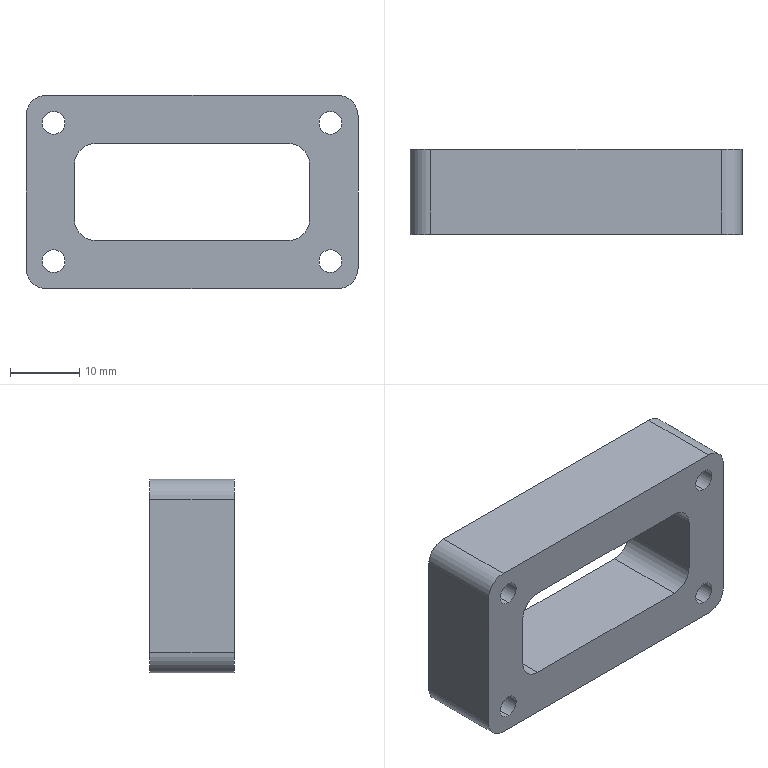Part | SolidWorks | features Extrusion 1 | 1 solid | 26 faces | box 48 x 12.25 x 28 mm | volume 10214 mm3 | cylinder 16 | plane 10 | commonest cylinder face diameters 3.3 x8 6 x8
STEP:
#1=CARTESIAN_POINT('',(20.,12.25,-11.65));
#2=VERTEX_POINT('',#1);
#3=CARTESIAN_POINT('',(20.,12.25,-8.35));
#4=VERTEX_POINT('',#3);
#5=CARTESIAN_POINT('',(20.,12.25,-10.));
#6=DIRECTION('',(0.,1.,0.));
#7=DIRECTION('',(0.,0.,1.));
#8=AXIS2_PLACEMENT_3D('',#5,#6,#7);
#9=CIRCLE('',#8,1.65);
#10=EDGE_CURVE('',#2,#4,#9,.T.);
#11=ORIENTED_EDGE('',*,*,#10,.T.);
#12=CARTESIAN_POINT('',(20.,0.,-8.35));
#13=VERTEX_POINT('',#12);
#14=CARTESIAN_POINT('',(20.,12.25,-8.35));
#15=DIRECTION('',(0.,-1.,0.));
#16=VECTOR('',#15,1000.);
#17=LINE('',#14,#16);
#18=EDGE_CURVE('',#4,#13,#17,.T.);
#19=ORIENTED_EDGE('',*,*,#18,.T.);
#20=CARTESIAN_POINT('',(20.,0.,-11.65));
#21=VERTEX_POINT('',#20);
#22=CARTESIAN_POINT('',(20.,0.,-10.));
#23=DIRECTION('',(0.,1.,0.));
#24=DIRECTION('',(0.,0.,1.));
#25=AXIS2_PLACEMENT_3D('',#22,#23,#24);
#26=CIRCLE('',#25,1.65);
#27=EDGE_CURVE('',#21,#13,#26,.T.);
#28=ORIENTED_EDGE('',*,*,#27,.F.);
#29=CARTESIAN_POINT('',(20.,12.25,-11.65));
#30=DIRECTION('',(0.,-1.,0.));
#31=VECTOR('',#30,1000.);
#32=LINE('',#29,#31);
#33=EDGE_CURVE('',#2,#21,#32,.T.);
#34=ORIENTED_EDGE('',*,*,#33,.F.);
#35=EDGE_LOOP('',(#11,#19,#28,#34));
#36=FACE_OUTER_BOUND('',#35,.T.);
#37=CARTESIAN_POINT('',(20.,12.25,-10.));
#38=DIRECTION('',(0.,-1.,0.));
#39=DIRECTION('',(0.,0.,-1.));
#40=AXIS2_PLACEMENT_3D('',#37,#38,#39);
#41=CYLINDRICAL_SURFACE('',#40,1.65);
#42=ADVANCED_FACE('',(#36),#41,.F.);
#43=CARTESIAN_POINT('',(20.,12.25,8.35));
#44=VERTEX_POINT('',#43);
#45=CARTESIAN_POINT('',(20.,12.25,11.65));
#46=VERTEX_POINT('',#45);
#47=CARTESIAN_POINT('',(20.,12.25,10.));
#48=DIRECTION('',(0.,1.,0.));
#49=DIRECTION('',(0.,0.,1.));
#50=AXIS2_PLACEMENT_3D('',#47,#48,#49);
#51=CIRCLE('',#50,1.65);
#52=EDGE_CURVE('',#44,#46,#51,.T.);
#53=ORIENTED_EDGE('',*,*,#52,.T.);
#54=CARTESIAN_POINT('',(20.,0.,11.65));
#55=VERTEX_POINT('',#54);
#56=CARTESIAN_POINT('',(20.,12.25,11.65));
#57=DIRECTION('',(0.,-1.,0.));
#58=VECTOR('',#57,1000.);
#59=LINE('',#56,#58);
#60=EDGE_CURVE('',#46,#55,#59,.T.);
#61=ORIENTED_EDGE('',*,*,#60,.T.);
#62=CARTESIAN_POINT('',(20.,0.,8.35));
#63=VERTEX_POINT('',#62);
#64=CARTESIAN_POINT('',(20.,0.,10.));
#65=DIRECTION('',(0.,1.,0.));
#66=DIRECTION('',(0.,0.,1.));
#67=AXIS2_PLACEMENT_3D('',#64,#65,#66);
#68=CIRCLE('',#67,1.65);
#69=EDGE_CURVE('',#63,#55,#68,.T.);
#70=ORIENTED_EDGE('',*,*,#69,.F.);
#71=CARTESIAN_POINT('',(20.,12.25,8.35));
#72=DIRECTION('',(0.,-1.,0.));
#73=VECTOR('',#72,1000.);
#74=LINE('',#71,#73);
#75=EDGE_CURVE('',#44,#63,#74,.T.);
#76=ORIENTED_EDGE('',*,*,#75,.F.);
#77=EDGE_LOOP('',(#53,#61,#70,#76));
#78=FACE_OUTER_BOUND('',#77,.T.);
#79=CARTESIAN_POINT('',(20.,12.25,10.));
#80=DIRECTION('',(0.,-1.,0.));
#81=DIRECTION('',(0.,0.,-1.));
#82=AXIS2_PLACEMENT_3D('',#79,#80,#81);
#83=CYLINDRICAL_SURFACE('',#82,1.65);
#84=ADVANCED_FACE('',(#78),#83,.F.);
#85=CARTESIAN_POINT('',(-20.,12.25,8.35));
#86=VERTEX_POINT('',#85);
#87=CARTESIAN_POINT('',(-20.,12.25,11.65));
#88=VERTEX_POINT('',#87);
#89=CARTESIAN_POINT('',(-20.,12.25,10.));
#90=DIRECTION('',(0.,1.,0.));
#91=DIRECTION('',(0.,0.,1.));
#92=AXIS2_PLACEMENT_3D('',#89,#90,#91);
#93=CIRCLE('',#92,1.65);
#94=EDGE_CURVE('',#86,#88,#93,.T.);
#95=ORIENTED_EDGE('',*,*,#94,.T.);
#96=CARTESIAN_POINT('',(-20.,0.,11.65));
#97=VERTEX_POINT('',#96);
#98=CARTESIAN_POINT('',(-20.,12.25,11.65));
#99=DIRECTION('',(0.,-1.,0.));
#100=VECTOR('',#99,1000.);
#101=LINE('',#98,#100);
#102=EDGE_CURVE('',#88,#97,#101,.T.);
#103=ORIENTED_EDGE('',*,*,#102,.T.);
#104=CARTESIAN_POINT('',(-20.,0.,8.35));
#105=VERTEX_POINT('',#104);
#106=CARTESIAN_POINT('',(-20.,0.,10.));
#107=DIRECTION('',(0.,1.,0.));
#108=DIRECTION('',(0.,0.,1.));
#109=AXIS2_PLACEMENT_3D('',#106,#107,#108);
#110=CIRCLE('',#109,1.65);
#111=EDGE_CURVE('',#105,#97,#110,.T.);
#112=ORIENTED_EDGE('',*,*,#111,.F.);
#113=CARTESIAN_POINT('',(-20.,12.25,8.35));
#114=DIRECTION('',(0.,-1.,0.));
#115=VECTOR('',#114,1000.);
#116=LINE('',#113,#115);
#117=EDGE_CURVE('',#86,#105,#116,.T.);
#118=ORIENTED_EDGE('',*,*,#117,.F.);
#119=EDGE_LOOP('',(#95,#103,#112,#118));
#120=FACE_OUTER_BOUND('',#119,.T.);
#121=CARTESIAN_POINT('',(-20.,12.25,10.));
#122=DIRECTION('',(0.,-1.,0.));
#123=DIRECTION('',(0.,0.,-1.));
#124=AXIS2_PLACEMENT_3D('',#121,#122,#123);
#125=CYLINDRICAL_SURFACE('',#124,1.65);
#126=ADVANCED_FACE('',(#120),#125,.F.);
#127=CARTESIAN_POINT('',(-20.,12.25,-11.65));
#128=VERTEX_POINT('',#127);
#129=CARTESIAN_POINT('',(-20.,12.25,-8.35));
#130=VERTEX_POINT('',#129);
#131=CARTESIAN_POINT('',(-20.,12.25,-10.));
#132=DIRECTION('',(0.,1.,0.));
#133=DIRECTION('',(0.,0.,1.));
#134=AXIS2_PLACEMENT_3D('',#131,#132,#133);
#135=CIRCLE('',#134,1.65);
#136=EDGE_CURVE('',#128,#130,#135,.T.);
#137=ORIENTED_EDGE('',*,*,#136,.T.);
#138=CARTESIAN_POINT('',(-20.,0.,-8.35));
#139=VERTEX_POINT('',#138);
#140=CARTESIAN_POINT('',(-20.,12.25,-8.35));
#141=DIRECTION('',(0.,-1.,0.));
#142=VECTOR('',#141,1000.);
#143=LINE('',#140,#142);
#144=EDGE_CURVE('',#130,#139,#143,.T.);
#145=ORIENTED_EDGE('',*,*,#144,.T.);
#146=CARTESIAN_POINT('',(-20.,0.,-11.65));
#147=VERTEX_POINT('',#146);
#148=CARTESIAN_POINT('',(-20.,0.,-10.));
#149=DIRECTION('',(0.,1.,0.));
#150=DIRECTION('',(0.,0.,1.));
#151=AXIS2_PLACEMENT_3D('',#148,#149,#150);
#152=CIRCLE('',#151,1.65);
#153=EDGE_CURVE('',#147,#139,#152,.T.);
#154=ORIENTED_EDGE('',*,*,#153,.F.);
#155=CARTESIAN_POINT('',(-20.,12.25,-11.65));
#156=DIRECTION('',(0.,-1.,0.));
#157=VECTOR('',#156,1000.);
#158=LINE('',#155,#157);
#159=EDGE_CURVE('',#128,#147,#158,.T.);
#160=ORIENTED_EDGE('',*,*,#159,.F.);
#161=EDGE_LOOP('',(#137,#145,#154,#160));
#162=FACE_OUTER_BOUND('',#161,.T.);
#163=CARTESIAN_POINT('',(-20.,12.25,-10.));
#164=DIRECTION('',(0.,-1.,0.));
#165=DIRECTION('',(0.,0.,-1.));
#166=AXIS2_PLACEMENT_3D('',#163,#164,#165);
#167=CYLINDRICAL_SURFACE('',#166,1.65);
#168=ADVANCED_FACE('',(#162),#167,.F.);
#169=ORIENTED_EDGE('',*,*,#10,.F.);
#170=CARTESIAN_POINT('',(20.,12.25,-10.));
#171=DIRECTION('',(0.,1.,0.));
#172=DIRECTION('',(0.,0.,1.));
#173=AXIS2_PLACEMENT_3D('',#170,#171,#172);
#174=CIRCLE('',#173,1.65);
#175=EDGE_CURVE('',#4,#2,#174,.T.);
#176=ORIENTED_EDGE('',*,*,#175,.F.);
#177=EDGE_LOOP('',(#169,#176));
#178=FACE_BOUND('',#177,.T.);
#179=ORIENTED_EDGE('',*,*,#52,.F.);
#180=CARTESIAN_POINT('',(20.,12.25,10.));
#181=DIRECTION('',(0.,1.,0.));
#182=DIRECTION('',(0.,0.,1.));
#183=AXIS2_PLACEMENT_3D('',#180,#181,#182);
#184=CIRCLE('',#183,1.65);
#185=EDGE_CURVE('',#46,#44,#184,.T.);
#186=ORIENTED_EDGE('',*,*,#185,.F.);
#187=EDGE_LOOP('',(#179,#186));
#188=FACE_BOUND('',#187,.T.);
#189=ORIENTED_EDGE('',*,*,#94,.F.);
#190=CARTESIAN_POINT('',(-20.,12.25,10.));
#191=DIRECTION('',(0.,1.,0.));
#192=DIRECTION('',(0.,0.,1.));
#193=AXIS2_PLACEMENT_3D('',#190,#191,#192);
#194=CIRCLE('',#193,1.65);
#195=EDGE_CURVE('',#88,#86,#194,.T.);
#196=ORIENTED_EDGE('',*,*,#195,.F.);
#197=EDGE_LOOP('',(#189,#196));
#198=FACE_BOUND('',#197,.T.);
#199=ORIENTED_EDGE('',*,*,#136,.F.);
#200=CARTESIAN_POINT('',(-20.,12.25,-10.));
#201=DIRECTION('',(0.,1.,0.));
#202=DIRECTION('',(0.,0.,1.));
#203=AXIS2_PLACEMENT_3D('',#200,#201,#202);
#204=CIRCLE('',#203,1.65);
#205=EDGE_CURVE('',#130,#128,#204,.T.);
#206=ORIENTED_EDGE('',*,*,#205,.F.);
#207=EDGE_LOOP('',(#199,#206));
#208=FACE_BOUND('',#207,.T.);
#209=CARTESIAN_POINT('',(21.,12.25,14.));
#210=VERTEX_POINT('',#209);
#211=CARTESIAN_POINT('',(24.,12.25,11.));
#212=VERTEX_POINT('',#211);
#213=CARTESIAN_POINT('',(21.,12.25,11.));
#214=DIRECTION('',(0.,1.,0.));
#215=DIRECTION('',(0.,0.,-1.));
#216=AXIS2_PLACEMENT_3D('',#213,#214,#215);
#217=CIRCLE('',#216,3.);
#218=EDGE_CURVE('',#210,#212,#217,.T.);
#219=ORIENTED_EDGE('',*,*,#218,.T.);
#220=CARTESIAN_POINT('',(24.,12.25,-11.));
#221=VERTEX_POINT('',#220);
#222=CARTESIAN_POINT('',(24.,12.25,11.));
#223=DIRECTION('',(0.,0.,-1.));
#224=VECTOR('',#223,1000.);
#225=LINE('',#222,#224);
#226=EDGE_CURVE('',#212,#221,#225,.T.);
#227=ORIENTED_EDGE('',*,*,#226,.T.);
#228=CARTESIAN_POINT('',(21.,12.25,-14.));
#229=VERTEX_POINT('',#228);
#230=CARTESIAN_POINT('',(21.,12.25,-11.));
#231=DIRECTION('',(0.,1.,0.));
#232=DIRECTION('',(0.,0.,-1.));
#233=AXIS2_PLACEMENT_3D('',#230,#231,#232);
#234=CIRCLE('',#233,3.);
#235=EDGE_CURVE('',#221,#229,#234,.T.);
#236=ORIENTED_EDGE('',*,*,#235,.T.);
#237=CARTESIAN_POINT('',(-21.,12.25,-14.));
#238=VERTEX_POINT('',#237);
#239=CARTESIAN_POINT('',(-21.,12.25,-14.));
#240=DIRECTION('',(-1.,0.,0.));
#241=VECTOR('',#240,1000.);
#242=LINE('',#239,#241);
#243=EDGE_CURVE('',#229,#238,#242,.T.);
#244=ORIENTED_EDGE('',*,*,#243,.T.);
#245=CARTESIAN_POINT('',(-24.,12.25,-11.));
#246=VERTEX_POINT('',#245);
#247=CARTESIAN_POINT('',(-21.,12.25,-11.));
#248=DIRECTION('',(0.,1.,0.));
#249=DIRECTION('',(0.,0.,-1.));
#250=AXIS2_PLACEMENT_3D('',#247,#248,#249);
#251=CIRCLE('',#250,3.);
#252=EDGE_CURVE('',#238,#246,#251,.T.);
#253=ORIENTED_EDGE('',*,*,#252,.T.);
#254=CARTESIAN_POINT('',(-24.,12.25,11.));
#255=VERTEX_POINT('',#254);
#256=CARTESIAN_POINT('',(-24.,12.25,11.));
#257=DIRECTION('',(0.,0.,1.));
#258=VECTOR('',#257,1000.);
#259=LINE('',#256,#258);
#260=EDGE_CURVE('',#246,#255,#259,.T.);
#261=ORIENTED_EDGE('',*,*,#260,.T.);
#262=CARTESIAN_POINT('',(-21.,12.25,14.));
#263=VERTEX_POINT('',#262);
#264=CARTESIAN_POINT('',(-21.,12.25,11.));
#265=DIRECTION('',(0.,1.,0.));
#266=DIRECTION('',(0.,0.,1.));
#267=AXIS2_PLACEMENT_3D('',#264,#265,#266);
#268=CIRCLE('',#267,3.);
#269=EDGE_CURVE('',#255,#263,#268,.T.);
#270=ORIENTED_EDGE('',*,*,#269,.T.);
#271=CARTESIAN_POINT('',(-21.,12.25,14.));
#272=DIRECTION('',(1.,0.,0.));
#273=VECTOR('',#272,1000.);
#274=LINE('',#271,#273);
#275=EDGE_CURVE('',#263,#210,#274,.T.);
#276=ORIENTED_EDGE('',*,*,#275,.T.);
#277=EDGE_LOOP('',(#219,#227,#236,#244,#253,#261,#270,#276));
#278=FACE_OUTER_BOUND('',#277,.T.);
#279=CARTESIAN_POINT('',(17.,12.25,-4.));
#280=VERTEX_POINT('',#279);
#281=CARTESIAN_POINT('',(14.,12.25,-7.));
#282=VERTEX_POINT('',#281);
#283=CARTESIAN_POINT('',(14.,12.25,-4.));
#284=DIRECTION('',(0.,1.,0.));
#285=DIRECTION('',(0.,0.,-1.));
#286=AXIS2_PLACEMENT_3D('',#283,#284,#285);
#287=CIRCLE('',#286,3.);
#288=EDGE_CURVE('',#280,#282,#287,.T.);
#289=ORIENTED_EDGE('',*,*,#288,.F.);
#290=CARTESIAN_POINT('',(17.,12.25,4.));
#291=VERTEX_POINT('',#290);
#292=CARTESIAN_POINT('',(17.,12.25,4.));
#293=DIRECTION('',(0.,0.,-1.));
#294=VECTOR('',#293,1000.);
#295=LINE('',#292,#294);
#296=EDGE_CURVE('',#291,#280,#295,.T.);
#297=ORIENTED_EDGE('',*,*,#296,.F.);
#298=CARTESIAN_POINT('',(14.,12.25,7.));
#299=VERTEX_POINT('',#298);
#300=CARTESIAN_POINT('',(14.,12.25,4.));
#301=DIRECTION('',(0.,1.,0.));
#302=DIRECTION('',(0.,0.,-1.));
#303=AXIS2_PLACEMENT_3D('',#300,#301,#302);
#304=CIRCLE('',#303,3.);
#305=EDGE_CURVE('',#299,#291,#304,.T.);
#306=ORIENTED_EDGE('',*,*,#305,.F.);
#307=CARTESIAN_POINT('',(-14.,12.25,7.));
#308=VERTEX_POINT('',#307);
#309=CARTESIAN_POINT('',(-14.,12.25,7.));
#310=DIRECTION('',(1.,0.,0.));
#311=VECTOR('',#310,1000.);
#312=LINE('',#309,#311);
#313=EDGE_CURVE('',#308,#299,#312,.T.);
#314=ORIENTED_EDGE('',*,*,#313,.F.);
#315=CARTESIAN_POINT('',(-17.,12.25,4.));
#316=VERTEX_POINT('',#315);
#317=CARTESIAN_POINT('',(-14.,12.25,4.));
#318=DIRECTION('',(0.,1.,0.));
#319=DIRECTION('',(0.,0.,1.));
#320=AXIS2_PLACEMENT_3D('',#317,#318,#319);
#321=CIRCLE('',#320,3.);
#322=EDGE_CURVE('',#316,#308,#321,.T.);
#323=ORIENTED_EDGE('',*,*,#322,.F.);
#324=CARTESIAN_POINT('',(-17.,12.25,-4.));
#325=VERTEX_POINT('',#324);
#326=CARTESIAN_POINT('',(-17.,12.25,4.));
#327=DIRECTION('',(0.,0.,1.));
#328=VECTOR('',#327,1000.);
#329=LINE('',#326,#328);
#330=EDGE_CURVE('',#325,#316,#329,.T.);
#331=ORIENTED_EDGE('',*,*,#330,.F.);
#332=CARTESIAN_POINT('',(-14.,12.25,-7.));
#333=VERTEX_POINT('',#332);
#334=CARTESIAN_POINT('',(-14.,12.25,-4.));
#335=DIRECTION('',(0.,1.,0.));
#336=DIRECTION('',(0.,0.,-1.));
#337=AXIS2_PLACEMENT_3D('',#334,#335,#336);
#338=CIRCLE('',#337,3.);
#339=EDGE_CURVE('',#333,#325,#338,.T.);
#340=ORIENTED_EDGE('',*,*,#339,.F.);
#341=CARTESIAN_POINT('',(-14.,12.25,-7.));
#342=DIRECTION('',(-1.,0.,0.));
#343=VECTOR('',#342,1000.);
#344=LINE('',#341,#343);
#345=EDGE_CURVE('',#282,#333,#344,.T.);
#346=ORIENTED_EDGE('',*,*,#345,.F.);
#347=EDGE_LOOP('',(#289,#297,#306,#314,#323,#331,#340,#346));
#348=FACE_BOUND('',#347,.T.);
#349=CARTESIAN_POINT('',(21.,12.25,11.));
#350=DIRECTION('',(0.,-1.,0.));
#351=DIRECTION('',(0.,0.,-1.));
#352=AXIS2_PLACEMENT_3D('',#349,#350,#351);
#353=PLANE('',#352);
#354=ADVANCED_FACE('',(#178,#188,#198,#208,#278,#348),#353,.F.);
#355=ORIENTED_EDGE('',*,*,#69,.T.);
#356=CARTESIAN_POINT('',(20.,0.,10.));
#357=DIRECTION('',(0.,1.,0.));
#358=DIRECTION('',(0.,0.,1.));
#359=AXIS2_PLACEMENT_3D('',#356,#357,#358);
#360=CIRCLE('',#359,1.65);
#361=EDGE_CURVE('',#55,#63,#360,.T.);
#362=ORIENTED_EDGE('',*,*,#361,.T.);
#363=EDGE_LOOP('',(#355,#362));
#364=FACE_BOUND('',#363,.T.);
#365=ORIENTED_EDGE('',*,*,#153,.T.);
#366=CARTESIAN_POINT('',(-20.,0.,-10.));
#367=DIRECTION('',(0.,1.,0.));
#368=DIRECTION('',(0.,0.,1.));
#369=AXIS2_PLACEMENT_3D('',#366,#367,#368);
#370=CIRCLE('',#369,1.65);
#371=EDGE_CURVE('',#139,#147,#370,.T.);
#372=ORIENTED_EDGE('',*,*,#371,.T.);
#373=EDGE_LOOP('',(#365,#372));
#374=FACE_BOUND('',#373,.T.);
#375=CARTESIAN_POINT('',(21.,0.,14.));
#376=VERTEX_POINT('',#375);
#377=CARTESIAN_POINT('',(24.,0.,11.));
#378=VERTEX_POINT('',#377);
#379=CARTESIAN_POINT('',(21.,0.,11.));
#380=DIRECTION('',(0.,1.,0.));
#381=DIRECTION('',(0.,0.,-1.));
#382=AXIS2_PLACEMENT_3D('',#379,#380,#381);
#383=CIRCLE('',#382,3.);
#384=EDGE_CURVE('',#376,#378,#383,.T.);
#385=ORIENTED_EDGE('',*,*,#384,.F.);
#386=CARTESIAN_POINT('',(-21.,0.,14.));
#387=VERTEX_POINT('',#386);
#388=CARTESIAN_POINT('',(-21.,0.,14.));
#389=DIRECTION('',(1.,0.,0.));
#390=VECTOR('',#389,1000.);
#391=LINE('',#388,#390);
#392=EDGE_CURVE('',#387,#376,#391,.T.);
#393=ORIENTED_EDGE('',*,*,#392,.F.);
#394=CARTESIAN_POINT('',(-24.,0.,11.));
#395=VERTEX_POINT('',#394);
#396=CARTESIAN_POINT('',(-21.,0.,11.));
#397=DIRECTION('',(0.,1.,0.));
#398=DIRECTION('',(0.,0.,1.));
#399=AXIS2_PLACEMENT_3D('',#396,#397,#398);
#400=CIRCLE('',#399,3.);
#401=EDGE_CURVE('',#395,#387,#400,.T.);
#402=ORIENTED_EDGE('',*,*,#401,.F.);
#403=CARTESIAN_POINT('',(-24.,0.,-11.));
#404=VERTEX_POINT('',#403);
#405=CARTESIAN_POINT('',(-24.,0.,11.));
#406=DIRECTION('',(0.,0.,1.));
#407=VECTOR('',#406,1000.);
#408=LINE('',#405,#407);
#409=EDGE_CURVE('',#404,#395,#408,.T.);
#410=ORIENTED_EDGE('',*,*,#409,.F.);
#411=CARTESIAN_POINT('',(-21.,0.,-14.));
#412=VERTEX_POINT('',#411);
#413=CARTESIAN_POINT('',(-21.,0.,-11.));
#414=DIRECTION('',(0.,1.,0.));
#415=DIRECTION('',(0.,0.,-1.));
#416=AXIS2_PLACEMENT_3D('',#413,#414,#415);
#417=CIRCLE('',#416,3.);
#418=EDGE_CURVE('',#412,#404,#417,.T.);
#419=ORIENTED_EDGE('',*,*,#418,.F.);
#420=CARTESIAN_POINT('',(21.,0.,-14.));
#421=VERTEX_POINT('',#420);
#422=CARTESIAN_POINT('',(-21.,0.,-14.));
#423=DIRECTION('',(-1.,0.,0.));
#424=VECTOR('',#423,1000.);
#425=LINE('',#422,#424);
#426=EDGE_CURVE('',#421,#412,#425,.T.);
#427=ORIENTED_EDGE('',*,*,#426,.F.);
#428=CARTESIAN_POINT('',(24.,0.,-11.));
#429=VERTEX_POINT('',#428);
#430=CARTESIAN_POINT('',(21.,0.,-11.));
#431=DIRECTION('',(0.,1.,0.));
#432=DIRECTION('',(0.,0.,-1.));
#433=AXIS2_PLACEMENT_3D('',#430,#431,#432);
#434=CIRCLE('',#433,3.);
#435=EDGE_CURVE('',#429,#421,#434,.T.);
#436=ORIENTED_EDGE('',*,*,#435,.F.);
#437=CARTESIAN_POINT('',(24.,0.,11.));
#438=DIRECTION('',(0.,0.,-1.));
#439=VECTOR('',#438,1000.);
#440=LINE('',#437,#439);
#441=EDGE_CURVE('',#378,#429,#440,.T.);
#442=ORIENTED_EDGE('',*,*,#441,.F.);
#443=EDGE_LOOP('',(#385,#393,#402,#410,#419,#427,#436,#442));
#444=FACE_OUTER_BOUND('',#443,.T.);
#445=ORIENTED_EDGE('',*,*,#111,.T.);
#446=CARTESIAN_POINT('',(-20.,0.,10.));
#447=DIRECTION('',(0.,1.,0.));
#448=DIRECTION('',(0.,0.,1.));
#449=AXIS2_PLACEMENT_3D('',#446,#447,#448);
#450=CIRCLE('',#449,1.65);
#451=EDGE_CURVE('',#97,#105,#450,.T.);
#452=ORIENTED_EDGE('',*,*,#451,.T.);
#453=EDGE_LOOP('',(#445,#452));
#454=FACE_BOUND('',#453,.T.);
#455=ORIENTED_EDGE('',*,*,#27,.T.);
#456=CARTESIAN_POINT('',(20.,0.,-10.));
#457=DIRECTION('',(0.,1.,0.));
#458=DIRECTION('',(0.,0.,1.));
#459=AXIS2_PLACEMENT_3D('',#456,#457,#458);
#460=CIRCLE('',#459,1.65);
#461=EDGE_CURVE('',#13,#21,#460,.T.);
#462=ORIENTED_EDGE('',*,*,#461,.T.);
#463=EDGE_LOOP('',(#455,#462));
#464=FACE_BOUND('',#463,.T.);
#465=CARTESIAN_POINT('',(17.,0.,4.));
#466=VERTEX_POINT('',#465);
#467=CARTESIAN_POINT('',(17.,0.,-4.));
#468=VERTEX_POINT('',#467);
#469=CARTESIAN_POINT('',(17.,0.,4.));
#470=DIRECTION('',(0.,0.,-1.));
#471=VECTOR('',#470,1000.);
#472=LINE('',#469,#471);
#473=EDGE_CURVE('',#466,#468,#472,.T.);
#474=ORIENTED_EDGE('',*,*,#473,.T.);
#475=CARTESIAN_POINT('',(14.,0.,-7.));
#476=VERTEX_POINT('',#475);
#477=CARTESIAN_POINT('',(14.,0.,-4.));
#478=DIRECTION('',(0.,1.,0.));
#479=DIRECTION('',(0.,0.,-1.));
#480=AXIS2_PLACEMENT_3D('',#477,#478,#479);
#481=CIRCLE('',#480,3.);
#482=EDGE_CURVE('',#468,#476,#481,.T.);
#483=ORIENTED_EDGE('',*,*,#482,.T.);
#484=CARTESIAN_POINT('',(-14.,0.,-7.));
#485=VERTEX_POINT('',#484);
#486=CARTESIAN_POINT('',(-14.,0.,-7.));
#487=DIRECTION('',(-1.,0.,0.));
#488=VECTOR('',#487,1000.);
#489=LINE('',#486,#488);
#490=EDGE_CURVE('',#476,#485,#489,.T.);
#491=ORIENTED_EDGE('',*,*,#490,.T.);
#492=CARTESIAN_POINT('',(-17.,0.,-4.));
#493=VERTEX_POINT('',#492);
#494=CARTESIAN_POINT('',(-14.,0.,-4.));
#495=DIRECTION('',(0.,1.,0.));
#496=DIRECTION('',(0.,0.,-1.));
#497=AXIS2_PLACEMENT_3D('',#494,#495,#496);
#498=CIRCLE('',#497,3.);
#499=EDGE_CURVE('',#485,#493,#498,.T.);
#500=ORIENTED_EDGE('',*,*,#499,.T.);
#501=CARTESIAN_POINT('',(-17.,0.,4.));
#502=VERTEX_POINT('',#501);
#503=CARTESIAN_POINT('',(-17.,0.,4.));
#504=DIRECTION('',(0.,0.,1.));
#505=VECTOR('',#504,1000.);
#506=LINE('',#503,#505);
#507=EDGE_CURVE('',#493,#502,#506,.T.);
#508=ORIENTED_EDGE('',*,*,#507,.T.);
#509=CARTESIAN_POINT('',(-14.,0.,7.));
#510=VERTEX_POINT('',#509);
#511=CARTESIAN_POINT('',(-14.,0.,4.));
#512=DIRECTION('',(0.,1.,0.));
#513=DIRECTION('',(0.,0.,1.));
#514=AXIS2_PLACEMENT_3D('',#511,#512,#513);
#515=CIRCLE('',#514,3.);
#516=EDGE_CURVE('',#502,#510,#515,.T.);
#517=ORIENTED_EDGE('',*,*,#516,.T.);
#518=CARTESIAN_POINT('',(14.,0.,7.));
#519=VERTEX_POINT('',#518);
#520=CARTESIAN_POINT('',(-14.,0.,7.));
#521=DIRECTION('',(1.,0.,0.));
#522=VECTOR('',#521,1000.);
#523=LINE('',#520,#522);
#524=EDGE_CURVE('',#510,#519,#523,.T.);
#525=ORIENTED_EDGE('',*,*,#524,.T.);
#526=CARTESIAN_POINT('',(14.,0.,4.));
#527=DIRECTION('',(0.,1.,0.));
#528=DIRECTION('',(0.,0.,-1.));
#529=AXIS2_PLACEMENT_3D('',#526,#527,#528);
#530=CIRCLE('',#529,3.);
#531=EDGE_CURVE('',#519,#466,#530,.T.);
#532=ORIENTED_EDGE('',*,*,#531,.T.);
#533=EDGE_LOOP('',(#474,#483,#491,#500,#508,#517,#525,#532));
#534=FACE_BOUND('',#533,.T.);
#535=CARTESIAN_POINT('',(21.,0.,11.));
#536=DIRECTION('',(0.,-1.,0.));
#537=DIRECTION('',(0.,0.,-1.));
#538=AXIS2_PLACEMENT_3D('',#535,#536,#537);
#539=PLANE('',#538);
#540=ADVANCED_FACE('',(#364,#374,#444,#454,#464,#534),#539,.T.);
#541=ORIENTED_EDGE('',*,*,#384,.T.);
#542=CARTESIAN_POINT('',(24.,12.25,11.));
#543=DIRECTION('',(0.,-1.,0.));
#544=VECTOR('',#543,1000.);
#545=LINE('',#542,#544);
#546=EDGE_CURVE('',#212,#378,#545,.T.);
#547=ORIENTED_EDGE('',*,*,#546,.F.);
#548=ORIENTED_EDGE('',*,*,#218,.F.);
#549=CARTESIAN_POINT('',(21.,12.25,14.));
#550=DIRECTION('',(0.,-1.,0.));
#551=VECTOR('',#550,1000.);
#552=LINE('',#549,#551);
#553=EDGE_CURVE('',#210,#376,#552,.T.);
#554=ORIENTED_EDGE('',*,*,#553,.T.);
#555=EDGE_LOOP('',(#541,#547,#548,#554));
#556=FACE_OUTER_BOUND('',#555,.T.);
#557=CARTESIAN_POINT('',(21.,12.25,11.));
#558=DIRECTION('',(0.,-1.,0.));
#559=DIRECTION('',(0.,0.,-1.));
#560=AXIS2_PLACEMENT_3D('',#557,#558,#559);
#561=CYLINDRICAL_SURFACE('',#560,3.);
#562=ADVANCED_FACE('',(#556),#561,.T.);
#563=ORIENTED_EDGE('',*,*,#441,.T.);
#564=CARTESIAN_POINT('',(24.,12.25,-11.));
#565=DIRECTION('',(0.,-1.,0.));
#566=VECTOR('',#565,1000.);
#567=LINE('',#564,#566);
#568=EDGE_CURVE('',#221,#429,#567,.T.);
#569=ORIENTED_EDGE('',*,*,#568,.F.);
#570=ORIENTED_EDGE('',*,*,#226,.F.);
#571=ORIENTED_EDGE('',*,*,#546,.T.);
#572=EDGE_LOOP('',(#563,#569,#570,#571));
#573=FACE_OUTER_BOUND('',#572,.T.);
#574=CARTESIAN_POINT('',(24.,12.25,11.));
#575=DIRECTION('',(-1.,0.,0.));
#576=DIRECTION('',(0.,0.,1.));
#577=AXIS2_PLACEMENT_3D('',#574,#575,#576);
#578=PLANE('',#577);
#579=ADVANCED_FACE('',(#573),#578,.F.);
#580=ORIENTED_EDGE('',*,*,#435,.T.);
#581=CARTESIAN_POINT('',(21.,12.25,-14.));
#582=DIRECTION('',(0.,-1.,0.));
#583=VECTOR('',#582,1000.);
#584=LINE('',#581,#583);
#585=EDGE_CURVE('',#229,#421,#584,.T.);
#586=ORIENTED_EDGE('',*,*,#585,.F.);
#587=ORIENTED_EDGE('',*,*,#235,.F.);
#588=ORIENTED_EDGE('',*,*,#568,.T.);
#589=EDGE_LOOP('',(#580,#586,#587,#588));
#590=FACE_OUTER_BOUND('',#589,.T.);
#591=CARTESIAN_POINT('',(21.,12.25,-11.));
#592=DIRECTION('',(0.,-1.,0.));
#593=DIRECTION('',(0.,0.,-1.));
#594=AXIS2_PLACEMENT_3D('',#591,#592,#593);
#595=CYLINDRICAL_SURFACE('',#594,3.);
#596=ADVANCED_FACE('',(#590),#595,.T.);
#597=ORIENTED_EDGE('',*,*,#426,.T.);
#598=CARTESIAN_POINT('',(-21.,12.25,-14.));
#599=DIRECTION('',(0.,-1.,0.));
#600=VECTOR('',#599,1000.);
#601=LINE('',#598,#600);
#602=EDGE_CURVE('',#238,#412,#601,.T.);
#603=ORIENTED_EDGE('',*,*,#602,.F.);
#604=ORIENTED_EDGE('',*,*,#243,.F.);
#605=ORIENTED_EDGE('',*,*,#585,.T.);
#606=EDGE_LOOP('',(#597,#603,#604,#605));
#607=FACE_OUTER_BOUND('',#606,.T.);
#608=CARTESIAN_POINT('',(-21.,12.25,-14.));
#609=DIRECTION('',(0.,0.,1.));
#610=DIRECTION('',(1.,0.,0.));
#611=AXIS2_PLACEMENT_3D('',#608,#609,#610);
#612=PLANE('',#611);
#613=ADVANCED_FACE('',(#607),#612,.F.);
#614=ORIENTED_EDGE('',*,*,#418,.T.);
#615=CARTESIAN_POINT('',(-24.,12.25,-11.));
#616=DIRECTION('',(0.,-1.,0.));
#617=VECTOR('',#616,1000.);
#618=LINE('',#615,#617);
#619=EDGE_CURVE('',#246,#404,#618,.T.);
#620=ORIENTED_EDGE('',*,*,#619,.F.);
#621=ORIENTED_EDGE('',*,*,#252,.F.);
#622=ORIENTED_EDGE('',*,*,#602,.T.);
#623=EDGE_LOOP('',(#614,#620,#621,#622));
#624=FACE_OUTER_BOUND('',#623,.T.);
#625=CARTESIAN_POINT('',(-21.,12.25,-11.));
#626=DIRECTION('',(0.,-1.,0.));
#627=DIRECTION('',(0.,0.,-1.));
#628=AXIS2_PLACEMENT_3D('',#625,#626,#627);
#629=CYLINDRICAL_SURFACE('',#628,3.);
#630=ADVANCED_FACE('',(#624),#629,.T.);
#631=ORIENTED_EDGE('',*,*,#409,.T.);
#632=CARTESIAN_POINT('',(-24.,12.25,11.));
#633=DIRECTION('',(0.,-1.,0.));
#634=VECTOR('',#633,1000.);
#635=LINE('',#632,#634);
#636=EDGE_CURVE('',#255,#395,#635,.T.);
#637=ORIENTED_EDGE('',*,*,#636,.F.);
#638=ORIENTED_EDGE('',*,*,#260,.F.);
#639=ORIENTED_EDGE('',*,*,#619,.T.);
#640=EDGE_LOOP('',(#631,#637,#638,#639));
#641=FACE_OUTER_BOUND('',#640,.T.);
#642=CARTESIAN_POINT('',(-24.,12.25,11.));
#643=DIRECTION('',(1.,0.,0.));
#644=DIRECTION('',(0.,0.,-1.));
#645=AXIS2_PLACEMENT_3D('',#642,#643,#644);
#646=PLANE('',#645);
#647=ADVANCED_FACE('',(#641),#646,.F.);
#648=ORIENTED_EDGE('',*,*,#401,.T.);
#649=CARTESIAN_POINT('',(-21.,12.25,14.));
#650=DIRECTION('',(0.,-1.,0.));
#651=VECTOR('',#650,1000.);
#652=LINE('',#649,#651);
#653=EDGE_CURVE('',#263,#387,#652,.T.);
#654=ORIENTED_EDGE('',*,*,#653,.F.);
#655=ORIENTED_EDGE('',*,*,#269,.F.);
#656=ORIENTED_EDGE('',*,*,#636,.T.);
#657=EDGE_LOOP('',(#648,#654,#655,#656));
#658=FACE_OUTER_BOUND('',#657,.T.);
#659=CARTESIAN_POINT('',(-21.,12.25,11.));
#660=DIRECTION('',(0.,-1.,0.));
#661=DIRECTION('',(0.,0.,-1.));
#662=AXIS2_PLACEMENT_3D('',#659,#660,#661);
#663=CYLINDRICAL_SURFACE('',#662,3.);
#664=ADVANCED_FACE('',(#658),#663,.T.);
#665=ORIENTED_EDGE('',*,*,#392,.T.);
#666=ORIENTED_EDGE('',*,*,#553,.F.);
#667=ORIENTED_EDGE('',*,*,#275,.F.);
#668=ORIENTED_EDGE('',*,*,#653,.T.);
#669=EDGE_LOOP('',(#665,#666,#667,#668));
#670=FACE_OUTER_BOUND('',#669,.T.);
#671=CARTESIAN_POINT('',(-21.,12.25,14.));
#672=DIRECTION('',(0.,0.,-1.));
#673=DIRECTION('',(-1.,0.,0.));
#674=AXIS2_PLACEMENT_3D('',#671,#672,#673);
#675=PLANE('',#674);
#676=ADVANCED_FACE('',(#670),#675,.F.);
#677=ORIENTED_EDGE('',*,*,#144,.F.);
#678=ORIENTED_EDGE('',*,*,#205,.T.);
#679=ORIENTED_EDGE('',*,*,#159,.T.);
#680=ORIENTED_EDGE('',*,*,#371,.F.);
#681=EDGE_LOOP('',(#677,#678,#679,#680));
#682=FACE_OUTER_BOUND('',#681,.T.);
#683=CARTESIAN_POINT('',(-20.,12.25,-10.));
#684=DIRECTION('',(0.,-1.,0.));
#685=DIRECTION('',(0.,0.,-1.));
#686=AXIS2_PLACEMENT_3D('',#683,#684,#685);
#687=CYLINDRICAL_SURFACE('',#686,1.65);
#688=ADVANCED_FACE('',(#682),#687,.F.);
#689=ORIENTED_EDGE('',*,*,#102,.F.);
#690=ORIENTED_EDGE('',*,*,#195,.T.);
#691=ORIENTED_EDGE('',*,*,#117,.T.);
#692=ORIENTED_EDGE('',*,*,#451,.F.);
#693=EDGE_LOOP('',(#689,#690,#691,#692));
#694=FACE_OUTER_BOUND('',#693,.T.);
#695=CARTESIAN_POINT('',(-20.,12.25,10.));
#696=DIRECTION('',(0.,-1.,0.));
#697=DIRECTION('',(0.,0.,-1.));
#698=AXIS2_PLACEMENT_3D('',#695,#696,#697);
#699=CYLINDRICAL_SURFACE('',#698,1.65);
#700=ADVANCED_FACE('',(#694),#699,.F.);
#701=ORIENTED_EDGE('',*,*,#60,.F.);
#702=ORIENTED_EDGE('',*,*,#185,.T.);
#703=ORIENTED_EDGE('',*,*,#75,.T.);
#704=ORIENTED_EDGE('',*,*,#361,.F.);
#705=EDGE_LOOP('',(#701,#702,#703,#704));
#706=FACE_OUTER_BOUND('',#705,.T.);
#707=CARTESIAN_POINT('',(20.,12.25,10.));
#708=DIRECTION('',(0.,-1.,0.));
#709=DIRECTION('',(0.,0.,-1.));
#710=AXIS2_PLACEMENT_3D('',#707,#708,#709);
#711=CYLINDRICAL_SURFACE('',#710,1.65);
#712=ADVANCED_FACE('',(#706),#711,.F.);
#713=ORIENTED_EDGE('',*,*,#18,.F.);
#714=ORIENTED_EDGE('',*,*,#175,.T.);
#715=ORIENTED_EDGE('',*,*,#33,.T.);
#716=ORIENTED_EDGE('',*,*,#461,.F.);
#717=EDGE_LOOP('',(#713,#714,#715,#716));
#718=FACE_OUTER_BOUND('',#717,.T.);
#719=CARTESIAN_POINT('',(20.,12.25,-10.));
#720=DIRECTION('',(0.,-1.,0.));
#721=DIRECTION('',(0.,0.,-1.));
#722=AXIS2_PLACEMENT_3D('',#719,#720,#721);
#723=CYLINDRICAL_SURFACE('',#722,1.65);
#724=ADVANCED_FACE('',(#718),#723,.F.);
#725=ORIENTED_EDGE('',*,*,#482,.F.);
#726=CARTESIAN_POINT('',(17.,12.25,-4.));
#727=DIRECTION('',(0.,-1.,0.));
#728=VECTOR('',#727,1000.);
#729=LINE('',#726,#728);
#730=EDGE_CURVE('',#280,#468,#729,.T.);
#731=ORIENTED_EDGE('',*,*,#730,.F.);
#732=ORIENTED_EDGE('',*,*,#288,.T.);
#733=CARTESIAN_POINT('',(14.,12.25,-7.));
#734=DIRECTION('',(0.,-1.,0.));
#735=VECTOR('',#734,1000.);
#736=LINE('',#733,#735);
#737=EDGE_CURVE('',#282,#476,#736,.T.);
#738=ORIENTED_EDGE('',*,*,#737,.T.);
#739=EDGE_LOOP('',(#725,#731,#732,#738));
#740=FACE_OUTER_BOUND('',#739,.T.);
#741=CARTESIAN_POINT('',(14.,12.25,-4.));
#742=DIRECTION('',(0.,-1.,0.));
#743=DIRECTION('',(0.,0.,-1.));
#744=AXIS2_PLACEMENT_3D('',#741,#742,#743);
#745=CYLINDRICAL_SURFACE('',#744,3.);
#746=ADVANCED_FACE('',(#740),#745,.F.);
#747=ORIENTED_EDGE('',*,*,#490,.F.);
#748=ORIENTED_EDGE('',*,*,#737,.F.);
#749=ORIENTED_EDGE('',*,*,#345,.T.);
#750=CARTESIAN_POINT('',(-14.,12.25,-7.));
#751=DIRECTION('',(0.,-1.,0.));
#752=VECTOR('',#751,1000.);
#753=LINE('',#750,#752);
#754=EDGE_CURVE('',#333,#485,#753,.T.);
#755=ORIENTED_EDGE('',*,*,#754,.T.);
#756=EDGE_LOOP('',(#747,#748,#749,#755));
#757=FACE_OUTER_BOUND('',#756,.T.);
#758=CARTESIAN_POINT('',(-14.,12.25,-7.));
#759=DIRECTION('',(0.,0.,1.));
#760=DIRECTION('',(1.,0.,0.));
#761=AXIS2_PLACEMENT_3D('',#758,#759,#760);
#762=PLANE('',#761);
#763=ADVANCED_FACE('',(#757),#762,.T.);
#764=ORIENTED_EDGE('',*,*,#499,.F.);
#765=ORIENTED_EDGE('',*,*,#754,.F.);
#766=ORIENTED_EDGE('',*,*,#339,.T.);
#767=CARTESIAN_POINT('',(-17.,12.25,-4.));
#768=DIRECTION('',(0.,-1.,0.));
#769=VECTOR('',#768,1000.);
#770=LINE('',#767,#769);
#771=EDGE_CURVE('',#325,#493,#770,.T.);
#772=ORIENTED_EDGE('',*,*,#771,.T.);
#773=EDGE_LOOP('',(#764,#765,#766,#772));
#774=FACE_OUTER_BOUND('',#773,.T.);
#775=CARTESIAN_POINT('',(-14.,12.25,-4.));
#776=DIRECTION('',(0.,-1.,0.));
#777=DIRECTION('',(0.,0.,-1.));
#778=AXIS2_PLACEMENT_3D('',#775,#776,#777);
#779=CYLINDRICAL_SURFACE('',#778,3.);
#780=ADVANCED_FACE('',(#774),#779,.F.);
#781=ORIENTED_EDGE('',*,*,#507,.F.);
#782=ORIENTED_EDGE('',*,*,#771,.F.);
#783=ORIENTED_EDGE('',*,*,#330,.T.);
#784=CARTESIAN_POINT('',(-17.,12.25,4.));
#785=DIRECTION('',(0.,-1.,0.));
#786=VECTOR('',#785,1000.);
#787=LINE('',#784,#786);
#788=EDGE_CURVE('',#316,#502,#787,.T.);
#789=ORIENTED_EDGE('',*,*,#788,.T.);
#790=EDGE_LOOP('',(#781,#782,#783,#789));
#791=FACE_OUTER_BOUND('',#790,.T.);
#792=CARTESIAN_POINT('',(-17.,12.25,4.));
#793=DIRECTION('',(1.,0.,0.));
#794=DIRECTION('',(0.,0.,-1.));
#795=AXIS2_PLACEMENT_3D('',#792,#793,#794);
#796=PLANE('',#795);
#797=ADVANCED_FACE('',(#791),#796,.T.);
#798=ORIENTED_EDGE('',*,*,#516,.F.);
#799=ORIENTED_EDGE('',*,*,#788,.F.);
#800=ORIENTED_EDGE('',*,*,#322,.T.);
#801=CARTESIAN_POINT('',(-14.,12.25,7.));
#802=DIRECTION('',(0.,-1.,0.));
#803=VECTOR('',#802,1000.);
#804=LINE('',#801,#803);
#805=EDGE_CURVE('',#308,#510,#804,.T.);
#806=ORIENTED_EDGE('',*,*,#805,.T.);
#807=EDGE_LOOP('',(#798,#799,#800,#806));
#808=FACE_OUTER_BOUND('',#807,.T.);
#809=CARTESIAN_POINT('',(-14.,12.25,4.));
#810=DIRECTION('',(0.,-1.,0.));
#811=DIRECTION('',(0.,0.,-1.));
#812=AXIS2_PLACEMENT_3D('',#809,#810,#811);
#813=CYLINDRICAL_SURFACE('',#812,3.);
#814=ADVANCED_FACE('',(#808),#813,.F.);
#815=ORIENTED_EDGE('',*,*,#524,.F.);
#816=ORIENTED_EDGE('',*,*,#805,.F.);
#817=ORIENTED_EDGE('',*,*,#313,.T.);
#818=CARTESIAN_POINT('',(14.,12.25,7.));
#819=DIRECTION('',(0.,-1.,0.));
#820=VECTOR('',#819,1000.);
#821=LINE('',#818,#820);
#822=EDGE_CURVE('',#299,#519,#821,.T.);
#823=ORIENTED_EDGE('',*,*,#822,.T.);
#824=EDGE_LOOP('',(#815,#816,#817,#823));
#825=FACE_OUTER_BOUND('',#824,.T.);
#826=CARTESIAN_POINT('',(-14.,12.25,7.));
#827=DIRECTION('',(0.,0.,-1.));
#828=DIRECTION('',(-1.,0.,0.));
#829=AXIS2_PLACEMENT_3D('',#826,#827,#828);
#830=PLANE('',#829);
#831=ADVANCED_FACE('',(#825),#830,.T.);
#832=ORIENTED_EDGE('',*,*,#531,.F.);
#833=ORIENTED_EDGE('',*,*,#822,.F.);
#834=ORIENTED_EDGE('',*,*,#305,.T.);
#835=CARTESIAN_POINT('',(17.,12.25,4.));
#836=DIRECTION('',(0.,-1.,0.));
#837=VECTOR('',#836,1000.);
#838=LINE('',#835,#837);
#839=EDGE_CURVE('',#291,#466,#838,.T.);
#840=ORIENTED_EDGE('',*,*,#839,.T.);
#841=EDGE_LOOP('',(#832,#833,#834,#840));
#842=FACE_OUTER_BOUND('',#841,.T.);
#843=CARTESIAN_POINT('',(14.,12.25,4.));
#844=DIRECTION('',(0.,-1.,0.));
#845=DIRECTION('',(0.,0.,-1.));
#846=AXIS2_PLACEMENT_3D('',#843,#844,#845);
#847=CYLINDRICAL_SURFACE('',#846,3.);
#848=ADVANCED_FACE('',(#842),#847,.F.);
#849=ORIENTED_EDGE('',*,*,#473,.F.);
#850=ORIENTED_EDGE('',*,*,#839,.F.);
#851=ORIENTED_EDGE('',*,*,#296,.T.);
#852=ORIENTED_EDGE('',*,*,#730,.T.);
#853=EDGE_LOOP('',(#849,#850,#851,#852));
#854=FACE_OUTER_BOUND('',#853,.T.);
#855=CARTESIAN_POINT('',(17.,12.25,4.));
#856=DIRECTION('',(-1.,0.,0.));
#857=DIRECTION('',(0.,0.,1.));
#858=AXIS2_PLACEMENT_3D('',#855,#856,#857);
#859=PLANE('',#858);
#860=ADVANCED_FACE('',(#854),#859,.T.);
#861=CLOSED_SHELL('',(#42,#84,#126,#168,#354,#540,#562,#579,#596,#613,#630,#647,#664,#676,#688,#700,#712,#724,#746,#763,#780,#797,#814,#831,#848,#860));
#862=MANIFOLD_SOLID_BREP('',#861);
#863=CARTESIAN_POINT('',(0.,0.,0.));
#864=DIRECTION('',(0.,0.,1.));
#865=DIRECTION('',(1.,0.,0.));
#866=AXIS2_PLACEMENT_3D('',#863,#864,#865);
#867=(LENGTH_UNIT()NAMED_UNIT(*)SI_UNIT(.MILLI.,.METRE.));
#868=UNCERTAINTY_MEASURE_WITH_UNIT(LENGTH_MEASURE(0.00001),#867,'','');
#869=(NAMED_UNIT(*)PLANE_ANGLE_UNIT()SI_UNIT($,.RADIAN.));
#870=(NAMED_UNIT(*)SI_UNIT($,.STERADIAN.)SOLID_ANGLE_UNIT());
#871=(GEOMETRIC_REPRESENTATION_CONTEXT(3)GLOBAL_UNCERTAINTY_ASSIGNED_CONTEXT((#868))GLOBAL_UNIT_ASSIGNED_CONTEXT((#867,#869,#870))REPRESENTATION_CONTEXT('',''));
#872=ADVANCED_BREP_SHAPE_REPRESENTATION('',(#862,#866),#871);